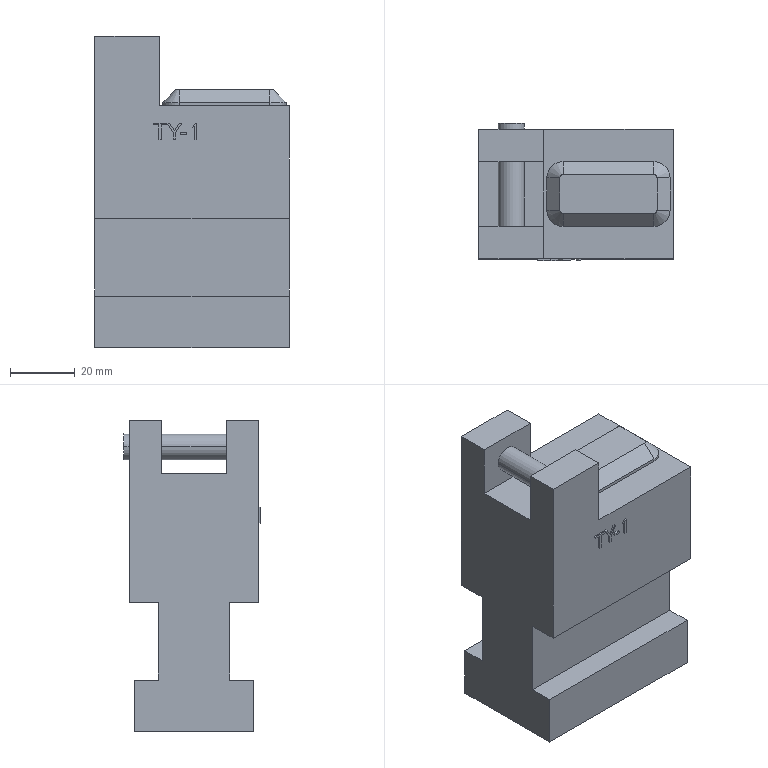Part | 1 solid | 74 faces | box 60 x 42.25 x 96.201 mm | volume 164955 mm3 | plane 60 | cylinder 8 | cone 4 | other 2 | commonest cylinder face diameters 8 x4 10 x4